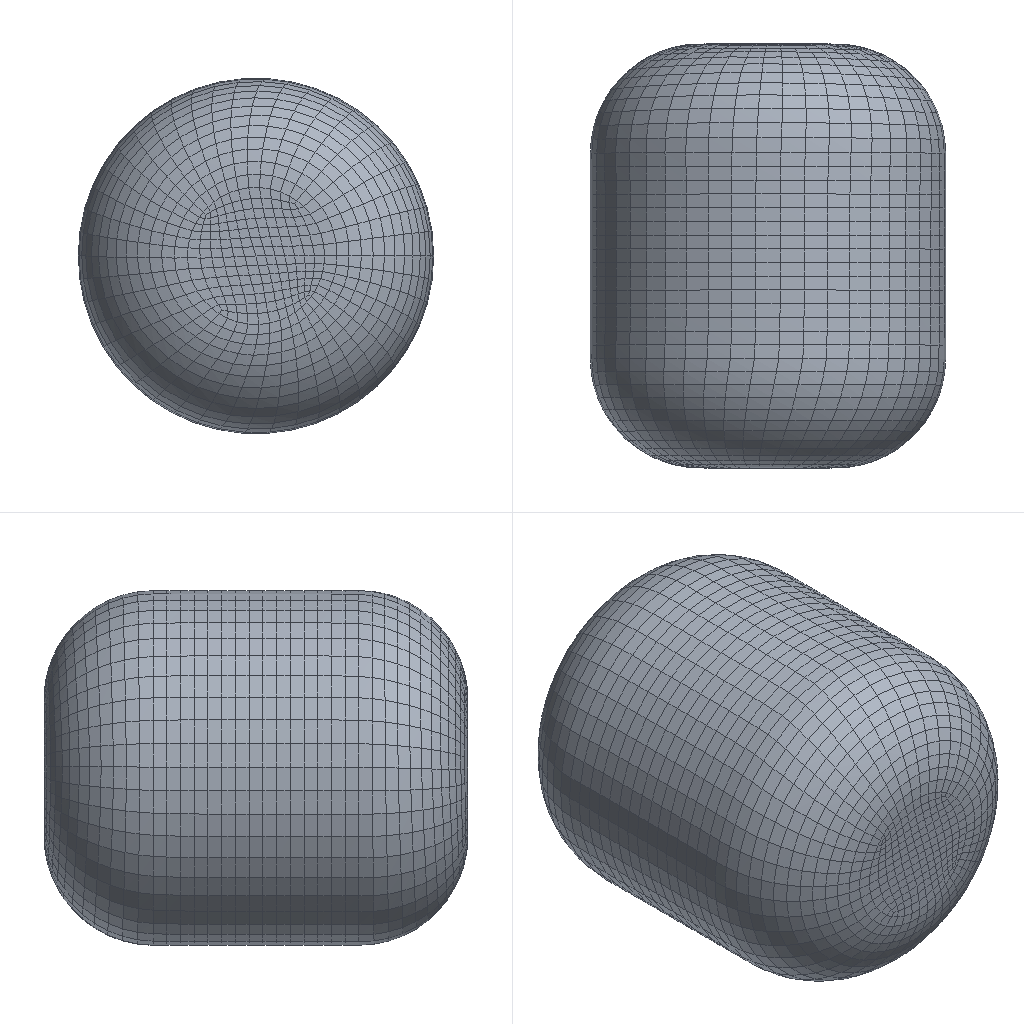Simulation study | abaqus
Set-up summary:
category,name,step,type,value,unit,region
solver,abaqus
solver,version,,,Abaqus/Explicit 2020
units,not stated in the deck,,not stated
analysis,deck,,transient,transient
load_step,Step-1,Step-1,transient
load_step,Step-2,Step-2,transient
load_step,requested,,,2
mesh,nodes,,,8345
mesh,elements,,,8126
element_type,S4,,shell,6726
element_type,R3D4,,rigid,1400
load,load commands in deck,,count,17
bc,support commands in deck,,count,70
material,NEI,,in results
material,PM,,in results
material,WAI,,in results
check,setup vs results,,match,"per instance, exact: element labels, types and connectivity; labels of the nodes the elements use; coordinates not compared"
Abaqus input file, long lists of numbers shortened:
*Heading
** Job name: Job-1 Model name: Model-1
** Generated by: Abaqus/CAE 2020
*Preprint, echo=NO, model=NO, history=NO, contact=NO
**
** PARTS
**
*Part, name=Part-4
*Node
      1,          -2.,          -2.,           0.
      2,  -1.6,          -2.,           0.
** (119 more lines like these left out)
*Element, type=R3D4
  1,   1,   2,  13,  12
  2,   2,   3,  14,  13
** (98 more lines like these left out)
*Node
    122,          -2.,           0.,           0.
*Nset, nset=Part-4-RefPt_, internal
122,
*Elset, elset=Part-4, generate
   1,  100,    1
*End Part
**
*Part, name=jiamian
*Node
      1,          1.5,          0.5,           0.
      2,   1.4,          0.5,           0.
** (339 more lines like these left out)
*Element, type=R3D4
  1,   1,   2,  33,  32
  2,   2,   3,  34,  33
** (298 more lines like these left out)
*Node
    342,         -1.5,           0.,           0.
*Nset, nset=jiamian-RefPt_, internal
342,
*Elset, elset=jiamian, generate
   1,  300,    1
*End Part
**
*Part, name=neinang
*Node
      1,           0.,          1.5,           0.
      2,          0.5,          1.5,           0.
** (2226 more lines like these left out)
*Element, type=S4
  1,  10,   9, 268, 265
  2,   9,   8, 269, 268
** (2224 more lines like these left out)
*Node
   2229,           0.,  -1.5,           0.
*Nset, nset=neinang-RefPt_, internal
2229,
*Nset, nset=_PickedSet2, internal, generate
    1,  2228,     1
*Elset, elset=_PickedSet2, internal, generate
    1,  2226,     1
*Nset, nset=fluidnode
 2229,
*Elset, elset=_Surf-1_SNEG, internal, generate
    1,  2226,     1
*Surface, type=ELEMENT, name=Surf-1
_Surf-1_SNEG, SNEG
*Elset, elset=_Surf-2_SPOS, internal, generate
    1,  2226,     1
*Surface, type=ELEMENT, name=Surf-2
_Surf-2_SPOS, SPOS
** Section: neinang
*Shell Section, elset=_PickedSet2, material=nei
0.001, 5
*End Part
**
*Part, name=pm
*Node
      1,           0.,   1.52,           0.
      2,          0.5,   1.52,           0.
** (2204 more lines like these left out)
*Element, type=S4
  1,  10,   9, 268, 265
  2,   9,   8, 269, 268
** (2202 more lines like these left out)
*Nset, nset=_PickedSet2, internal, generate
    1,  2206,     1
*Elset, elset=_PickedSet2, internal, generate
    1,  2204,     1
*Elset, elset=_Surf-1_SNEG, internal, generate
    1,  2204,     1
*Surface, type=ELEMENT, name=Surf-1
_Surf-1_SNEG, SNEG
*Elset, elset=_Surf-2_SPOS, internal, generate
    1,  2204,     1
*Surface, type=ELEMENT, name=Surf-2
_Surf-2_SPOS, SPOS
** Section: pm
*Shell Section, elset=_PickedSet2, material=pm
0.04, 5
*End Part
**
*Part, name=wainang
*Node
      1,           0.,   1.546,           0.
      2,          0.5,   1.546,           0.
** (2296 more lines like these left out)
*Element, type=S4
  1,  10,   9, 270, 267
  2,   9,   8, 271, 270
** (2294 more lines like these left out)
*Nset, nset=_PickedSet2, internal, generate
    1,  2298,     1
*Elset, elset=_PickedSet2, internal, generate
    1,  2296,     1
*Nset, nset=diquan
   5, 186, 187, 188, 189, 190, 191, 192, 193, 194, 195, 196, 197, 198, 199, 200
 201, 202, 203, 204, 205, 206, 207, 208, 209, 210, 211, 212, 213, 214, 215, 216
** (1 more lines like these left out)
*Elset, elset=diquan
 1521, 1534, 1547, 1560, 1573, 1586, 1599, 1612, 1625, 1638, 1651, 1664, 1677, 1690, 1703, 1716
 1729, 1742, 1755, 1768, 1781, 1794, 1807, 1832, 1845, 1858, 1871, 1884, 1897, 1910, 1923, 1936
** (4 more lines like these left out)
*Nset, nset=topmian
   1,   2,   7,   8,   9,  10,  11,  12,  13,  14,  15,  16,  17,  18,  19,  20
  21,  22,  23,  24,  25,  26,  27,  28,  29,  30,  31,  32,  33,  34,  35,  36
** (14 more lines like these left out)
*Elset, elset=topmian, generate
   1,  232,    1
*Elset, elset=_Surf-1_SNEG, internal, generate
    1,  2296,     1
*Surface, type=ELEMENT, name=Surf-1
_Surf-1_SNEG, SNEG
** Section: wainang
*Shell Section, elset=_PickedSet2, material=wai
0.01, 5
*End Part
**
**
** ASSEMBLY
**
*Assembly, name=Assembly
**
*Instance, name=neinang-1, part=neinang
*End Instance
**
*Instance, name=pm-1, part=pm
*End Instance
**
*Instance, name=wainang-1, part=wainang
*End Instance
**
*Instance, name=Part-4-1, part=Part-4
          0.,         1.56,           0.
          0.,         1.56,           0., 1.,         1.56,           0., 90.
*End Instance
**
*Instance, name=Part-4-2, part=Part-4
          0.,        -1.55,           0.
          0.,        -1.55,           0., 1.,        -1.55,           0., 90.
*End Instance
**
*Instance, name=jiamian-1, part=jiamian
          0.,           0.,          1.8
          0.,           0.,          1.8, 1.,           0.,          1.8, 90.
*End Instance
**
*Instance, name=jiamian-2, part=jiamian
          0.,           0.,         -1.8
          0.,           0.,         -1.8, 1.,           0.,         -1.8, 90.
*End Instance
**
*Instance, name=jiamian-3, part=jiamian
         1.8,           0.,           0.
         1.8,           0.,           0., 1.223, 0.5774, 0.5774,         120.
*End Instance
**
*Instance, name=jiamian-4, part=jiamian
        -1.8,           0.,           0.
        -1.8,           0.,           0., -2.377, 0.5774, 0.5774,         120.
*End Instance
**
*Nset, nset=_PickedSet34, internal, instance=Part-4-2
 122,
*Nset, nset=_PickedSet35, internal, instance=Part-4-1
 122,
*Nset, nset=_PickedSet37, internal, instance=jiamian-1
 342,
*Nset, nset=_PickedSet38, internal, instance=jiamian-3
 342,
*Nset, nset=_PickedSet39, internal, instance=jiamian-2
 342,
*Nset, nset=_PickedSet40, internal, instance=jiamian-4
 342,
*Elset, elset=_Surf-1_SNEG, internal, instance=neinang-1, generate
  233,  2026,     1
*Surface, type=ELEMENT, name=Surf-1
_Surf-1_SNEG, SNEG
*Rigid Body, ref node=Part-4-1.Part-4-RefPt_, elset=Part-4-1.Part-4
*Rigid Body, ref node=Part-4-2.Part-4-RefPt_, elset=Part-4-2.Part-4
*Rigid Body, ref node=jiamian-1.jiamian-RefPt_, elset=jiamian-1.jiamian
*Rigid Body, ref node=jiamian-2.jiamian-RefPt_, elset=jiamian-2.jiamian
*Rigid Body, ref node=jiamian-3.jiamian-RefPt_, elset=jiamian-3.jiamian
*Rigid Body, ref node=jiamian-4.jiamian-RefPt_, elset=jiamian-4.jiamian
** Constraint: Constraint-1
*Tie, name=Constraint-1, adjust=yes
neinang-1.Surf-2, pm-1.Surf-1
** Constraint: Constraint-2
*Tie, name=Constraint-2, adjust=yes
wainang-1.Surf-1, pm-1.Surf-2
*End Assembly
*Amplitude, name=Amp-1
             0.,              0.,             0.1,              1.
*Amplitude, name=Amp-2
             0.,              0.,              1.,              1.
**
** MATERIALS
**
*Material, name=nei
*Density
1440.,
*Elastic
 2e+08, 0.3
*Material, name=pm
*Density
15.,
*Elastic
 1.8e+07, 0.28
*Material, name=wai
*Density
980.,
*Elastic
 1.24e+10, 0.3
**
** INTERACTION PROPERTIES
**
*Surface Interaction, name=IntProp-1
*Friction
 0.12,
*Fluid Behavior, name=IntProp-2
*Molecular Weight
0.02879
*Capacity, type=POLYNOMIAL
 28.11,   0.001967,  4.802e-06, -1.966e-09,         0.
**
** PHYSICAL CONSTANTS
**
*Physical Constants, absolute zero=-273.15, universal gas=8.314
**
** INTERACTIONS
**
** Interaction: Int-1
*Contact, op=NEW
*Contact Inclusions, ALL EXTERIOR
*Contact Property Assignment
 ,  , IntProp-1
** ----------------------------------------------------------------
**
** STEP: Step-1
**
*Step, name=Step-1, nlgeom=YES
*Dynamic, Explicit
, 0.1
*Bulk Viscosity
0.06, 1.2
**
** BOUNDARY CONDITIONS
**
** Name: BC-1 Type: 对称/反对称/完全固定
*Boundary
_PickedSet34, ENCASTRE
** Name: BC-2 Type: 对称/反对称/完全固定
*Boundary
wainang-1.diquan, ENCASTRE
** Name: BC-3 Type: 位移/转角
*Boundary, amplitude=Amp-1
_PickedSet35, 1, 1
_PickedSet35, 2, 2, -2.7
_PickedSet35, 3, 3
_PickedSet35, 4, 4
_PickedSet35, 5, 5
_PickedSet35, 6, 6
** Name: BC-4 Type: 位移/转角
*Boundary, amplitude=Amp-1
_PickedSet37, 1, 1
_PickedSet37, 2, 2, -1.35
_PickedSet37, 3, 3, -0.3
_PickedSet37, 4, 4
_PickedSet37, 5, 5
_PickedSet37, 6, 6
** Name: BC-5 Type: 位移/转角
*Boundary, amplitude=Amp-1
_PickedSet38, 1, 1, -0.3
_PickedSet38, 2, 2, -1.35
_PickedSet38, 3, 3
_PickedSet38, 4, 4
_PickedSet38, 5, 5
_PickedSet38, 6, 6
** Name: BC-6 Type: 位移/转角
*Boundary, amplitude=Amp-1
_PickedSet39, 1, 1
_PickedSet39, 2, 2, -1.35
_PickedSet39, 3, 3, 0.3
_PickedSet39, 4, 4
_PickedSet39, 5, 5
_PickedSet39, 6, 6
** Name: BC-7 Type: 位移/转角
*Boundary, amplitude=Amp-1
_PickedSet40, 1, 1, 0.3
_PickedSet40, 2, 2, -1.35
_PickedSet40, 3, 3
_PickedSet40, 4, 4
_PickedSet40, 5, 5
_PickedSet40, 6, 6
** Name: BC-8 Type: 位移/转角
*Boundary, amplitude=Amp-1
wainang-1.topmian, 1, 1
wainang-1.topmian, 2, 2, -2.7
wainang-1.topmian, 3, 3
wainang-1.topmian, 4, 4
wainang-1.topmian, 5, 5
wainang-1.topmian, 6, 6
**
** OUTPUT REQUESTS
**
*Restart, write, number interval=1, time marks=NO
**
** FIELD OUTPUT: F-Output-1
**
*Output, field
*Node Output
A, RF, U, V
*Element Output, directions=YES
E, EVF, LE, MISES, PE, PEEQ, PEEQVAVG, PEVAVG, S, SVAVG
*Contact Output
CSTRESS,
**
** HISTORY OUTPUT: H-Output-1
**
*Output, history, variable=PRESELECT
*End Step
** ----------------------------------------------------------------
**
** STEP: Step-2
**
*Step, name=Step-2, nlgeom=YES
*Dynamic, Explicit
, 5.
*Bulk Viscosity
0.06, 1.2
**
** BOUNDARY CONDITIONS
**
** Name: BC-1 Type: 对称/反对称/完全固定
*Boundary, op=NEW
_PickedSet34, ENCASTRE
** Name: BC-2 Type: 对称/反对称/完全固定
*Boundary, op=NEW
wainang-1.diquan, ENCASTRE
** Name: BC-3 Type: 位移/转角
*Boundary, op=NEW, amplitude=Amp-2
_PickedSet35, 1, 1
_PickedSet35, 2, 2, 20.
_PickedSet35, 3, 3
_PickedSet35, 4, 4
_PickedSet35, 5, 5
_PickedSet35, 6, 6
** Name: BC-4 Type: 位移/转角
*Boundary, op=NEW, amplitude=Amp-2
_PickedSet37, 1, 1
_PickedSet37, 2, 2
_PickedSet37, 3, 3, 5.
_PickedSet37, 4, 4
_PickedSet37, 5, 5
_PickedSet37, 6, 6
** Name: BC-5 Type: 位移/转角
*Boundary, op=NEW, amplitude=Amp-2
_PickedSet38, 1, 1, 5.
_PickedSet38, 2, 2, -1.35
_PickedSet38, 3, 3
_PickedSet38, 4, 4
_PickedSet38, 5, 5
_PickedSet38, 6, 6
** Name: BC-6 Type: 位移/转角
*Boundary, op=NEW, amplitude=Amp-2
_PickedSet39, 1, 1
_PickedSet39, 2, 2
_PickedSet39, 3, 3, -5.
_PickedSet39, 4, 4
_PickedSet39, 5, 5
_PickedSet39, 6, 6
** Name: BC-7 Type: 位移/转角
*Boundary, op=NEW, amplitude=Amp-2
_PickedSet40, 1, 1, -5.
_PickedSet40, 2, 2
_PickedSet40, 3, 3
_PickedSet40, 4, 4
_PickedSet40, 5, 5
_PickedSet40, 6, 6
** Name: BC-8 Type: 位移/转角
*Boundary, op=NEW
**
** LOADS
**
** Name: Load-1   Type: Pressure
*Dsload
Surf-1, P, 0.05
**
** OUTPUT REQUESTS
**
*Restart, write, number interval=1, time marks=NO
**
** FIELD OUTPUT: F-Output-1
**
*Output, field
*Node Output
A, RF, U, V
*Element Output, directions=YES
E, EVF, LE, MISES, PE, PEEQ, PEEQVAVG, PEVAVG, S, SVAVG
*Contact Output
CSTRESS,
**
** HISTORY OUTPUT: H-Output-1
**
*Output, history, variable=PRESELECT
*End Step
Results summary:
result,step,Step-1,completed,increments=17792 time=0.1/0.1
result,step,Step-2,partial,increments=322336 time=1.813/5.0
result,analysis,,,transient
result,last_loadstep,,,2
result,primary field,,,"U, UR"
result,reaction total,,FX,-79401.664,model units
result,reaction total,,FY,246.711,model units
result,reaction total,,FZ,-80356.352,model units